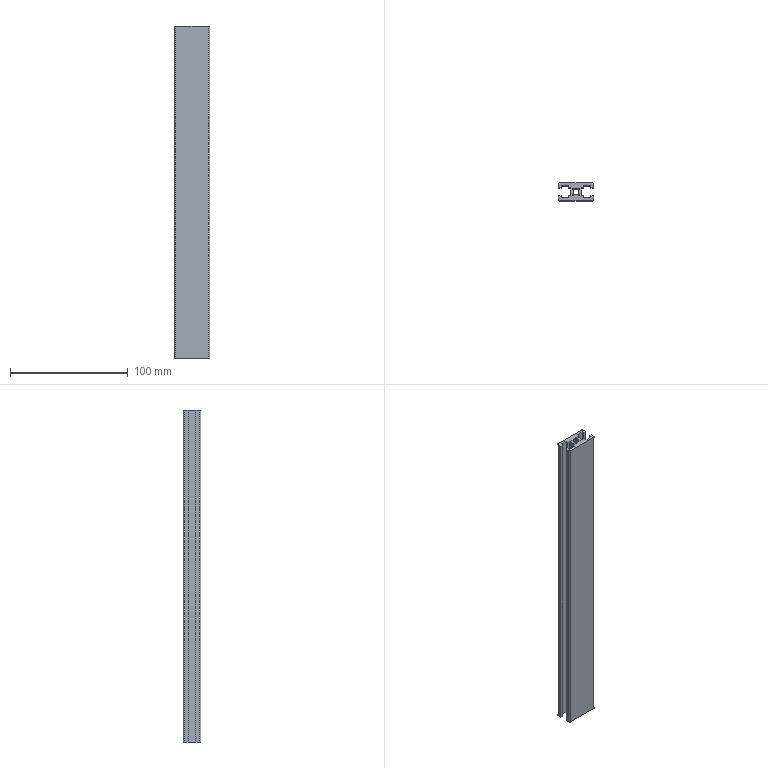Part | NX | features BREP 1 | 1 solid | 53 faces | box 30 x 15 x 282 mm | volume 68010 mm3 | plane 38 | cylinder 15 | commonest cylinder face diameters 1 x6 5 x5 2 x4